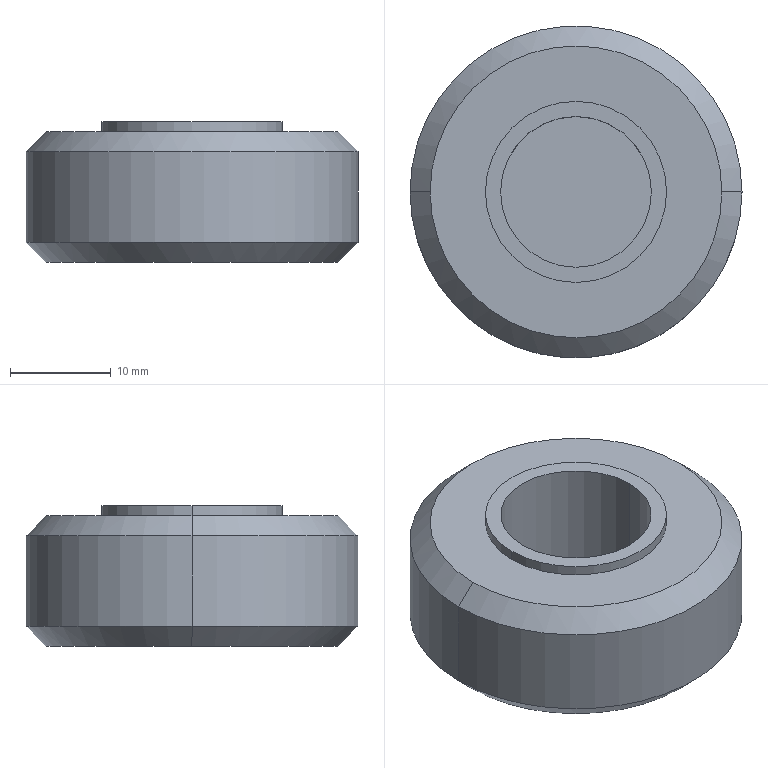Part | SolidWorks | features ICE 2, Chamfer 1, Extrusion 1 | 1 solid | 14 faces | box 33 x 33 x 14 mm | volume 9032 mm3 | cylinder 6 | cone 4 | plane 4 | commonest cylinder face diameters 15 x2 18 x2 33 x2
STEP:
#1=CARTESIAN_POINT('',(-14.5,0.,-3.));
#2=VERTEX_POINT('',#1);
#3=CARTESIAN_POINT('',(14.5,0.,-3.));
#4=VERTEX_POINT('',#3);
#5=CARTESIAN_POINT('',(0.,0.,-3.));
#6=DIRECTION('',(0.,0.,-1.));
#7=DIRECTION('',(-1.,0.,0.));
#8=AXIS2_PLACEMENT_3D('',#5,#6,#7);
#9=CIRCLE('',#8,14.5);
#10=EDGE_CURVE('',#2,#4,#9,.T.);
#11=ORIENTED_EDGE('',*,*,#10,.F.);
#12=CARTESIAN_POINT('',(-16.5,0.,-1.));
#13=VERTEX_POINT('',#12);
#14=CARTESIAN_POINT('',(-14.5,0.,-3.));
#15=DIRECTION('',(-0.7071,0.,0.7071));
#16=VECTOR('',#15,1000.);
#17=LINE('',#14,#16);
#18=EDGE_CURVE('',#2,#13,#17,.T.);
#19=ORIENTED_EDGE('',*,*,#18,.T.);
#20=CARTESIAN_POINT('',(16.5,0.,-1.));
#21=VERTEX_POINT('',#20);
#22=CARTESIAN_POINT('',(0.,0.,-1.));
#23=DIRECTION('',(0.,0.,1.));
#24=DIRECTION('',(-1.,0.,0.));
#25=AXIS2_PLACEMENT_3D('',#22,#23,#24);
#26=CIRCLE('',#25,16.5);
#27=EDGE_CURVE('',#21,#13,#26,.T.);
#28=ORIENTED_EDGE('',*,*,#27,.F.);
#29=CARTESIAN_POINT('',(14.5,0.,-3.));
#30=DIRECTION('',(0.7071,0.,0.7071));
#31=VECTOR('',#30,1000.);
#32=LINE('',#29,#31);
#33=EDGE_CURVE('',#4,#21,#32,.T.);
#34=ORIENTED_EDGE('',*,*,#33,.F.);
#35=EDGE_LOOP('',(#11,#19,#28,#34));
#36=FACE_OUTER_BOUND('',#35,.T.);
#37=CARTESIAN_POINT('',(0.,0.,-3.));
#38=DIRECTION('',(0.,0.,1.));
#39=DIRECTION('',(1.,0.,0.));
#40=AXIS2_PLACEMENT_3D('',#37,#38,#39);
#41=CONICAL_SURFACE('',#40,14.5,0.7854);
#42=ADVANCED_FACE('',(#36),#41,.T.);
#43=CARTESIAN_POINT('',(14.5,0.,10.));
#44=VERTEX_POINT('',#43);
#45=CARTESIAN_POINT('',(-14.5,0.,10.));
#46=VERTEX_POINT('',#45);
#47=CARTESIAN_POINT('',(0.,0.,10.));
#48=DIRECTION('',(0.,0.,1.));
#49=DIRECTION('',(1.,0.,0.));
#50=AXIS2_PLACEMENT_3D('',#47,#48,#49);
#51=CIRCLE('',#50,14.5);
#52=EDGE_CURVE('',#44,#46,#51,.T.);
#53=ORIENTED_EDGE('',*,*,#52,.F.);
#54=CARTESIAN_POINT('',(16.5,0.,8.));
#55=VERTEX_POINT('',#54);
#56=CARTESIAN_POINT('',(14.5,0.,10.));
#57=DIRECTION('',(0.7071,0.,-0.7071));
#58=VECTOR('',#57,1000.);
#59=LINE('',#56,#58);
#60=EDGE_CURVE('',#44,#55,#59,.T.);
#61=ORIENTED_EDGE('',*,*,#60,.T.);
#62=CARTESIAN_POINT('',(-16.5,0.,8.));
#63=VERTEX_POINT('',#62);
#64=CARTESIAN_POINT('',(0.,0.,8.));
#65=DIRECTION('',(0.,0.,-1.));
#66=DIRECTION('',(1.,0.,0.));
#67=AXIS2_PLACEMENT_3D('',#64,#65,#66);
#68=CIRCLE('',#67,16.5);
#69=EDGE_CURVE('',#63,#55,#68,.T.);
#70=ORIENTED_EDGE('',*,*,#69,.F.);
#71=CARTESIAN_POINT('',(-14.5,0.,10.));
#72=DIRECTION('',(-0.7071,0.,-0.7071));
#73=VECTOR('',#72,1000.);
#74=LINE('',#71,#73);
#75=EDGE_CURVE('',#46,#63,#74,.T.);
#76=ORIENTED_EDGE('',*,*,#75,.F.);
#77=EDGE_LOOP('',(#53,#61,#70,#76));
#78=FACE_OUTER_BOUND('',#77,.T.);
#79=CARTESIAN_POINT('',(0.,0.,10.));
#80=DIRECTION('',(0.,0.,-1.));
#81=DIRECTION('',(-1.,0.,0.));
#82=AXIS2_PLACEMENT_3D('',#79,#80,#81);
#83=CONICAL_SURFACE('',#82,14.5,0.7854);
#84=ADVANCED_FACE('',(#78),#83,.T.);
#85=CARTESIAN_POINT('',(9.,0.,11.));
#86=VERTEX_POINT('',#85);
#87=CARTESIAN_POINT('',(-9.,0.,11.));
#88=VERTEX_POINT('',#87);
#89=CARTESIAN_POINT('',(0.,0.,11.));
#90=DIRECTION('',(0.,0.,1.));
#91=DIRECTION('',(1.,0.,0.));
#92=AXIS2_PLACEMENT_3D('',#89,#90,#91);
#93=CIRCLE('',#92,9.);
#94=EDGE_CURVE('',#86,#88,#93,.T.);
#95=ORIENTED_EDGE('',*,*,#94,.F.);
#96=CARTESIAN_POINT('',(9.,0.,10.));
#97=VERTEX_POINT('',#96);
#98=CARTESIAN_POINT('',(9.,0.,11.));
#99=DIRECTION('',(0.,0.,-1.));
#100=VECTOR('',#99,1000.);
#101=LINE('',#98,#100);
#102=EDGE_CURVE('',#86,#97,#101,.T.);
#103=ORIENTED_EDGE('',*,*,#102,.T.);
#104=CARTESIAN_POINT('',(-9.,0.,10.));
#105=VERTEX_POINT('',#104);
#106=CARTESIAN_POINT('',(0.,0.,10.));
#107=DIRECTION('',(0.,0.,1.));
#108=DIRECTION('',(1.,0.,0.));
#109=AXIS2_PLACEMENT_3D('',#106,#107,#108);
#110=CIRCLE('',#109,9.);
#111=EDGE_CURVE('',#97,#105,#110,.T.);
#112=ORIENTED_EDGE('',*,*,#111,.T.);
#113=CARTESIAN_POINT('',(-9.,0.,11.));
#114=DIRECTION('',(0.,0.,-1.));
#115=VECTOR('',#114,1000.);
#116=LINE('',#113,#115);
#117=EDGE_CURVE('',#88,#105,#116,.T.);
#118=ORIENTED_EDGE('',*,*,#117,.F.);
#119=EDGE_LOOP('',(#95,#103,#112,#118));
#120=FACE_OUTER_BOUND('',#119,.T.);
#121=CARTESIAN_POINT('',(0.,0.,11.));
#122=DIRECTION('',(0.,0.,-1.));
#123=DIRECTION('',(-1.,0.,0.));
#124=AXIS2_PLACEMENT_3D('',#121,#122,#123);
#125=CYLINDRICAL_SURFACE('',#124,9.);
#126=ADVANCED_FACE('',(#120),#125,.T.);
#127=CARTESIAN_POINT('',(-7.5,0.,11.));
#128=VERTEX_POINT('',#127);
#129=CARTESIAN_POINT('',(7.5,0.,11.));
#130=VERTEX_POINT('',#129);
#131=CARTESIAN_POINT('',(0.,0.,11.));
#132=DIRECTION('',(0.,0.,1.));
#133=DIRECTION('',(1.,0.,0.));
#134=AXIS2_PLACEMENT_3D('',#131,#132,#133);
#135=CIRCLE('',#134,7.5);
#136=EDGE_CURVE('',#128,#130,#135,.T.);
#137=ORIENTED_EDGE('',*,*,#136,.T.);
#138=CARTESIAN_POINT('',(7.5,0.,0.));
#139=VERTEX_POINT('',#138);
#140=CARTESIAN_POINT('',(7.5,0.,10.));
#141=DIRECTION('',(0.,0.,-1.));
#142=VECTOR('',#141,1000.);
#143=LINE('',#140,#142);
#144=EDGE_CURVE('',#130,#139,#143,.T.);
#145=ORIENTED_EDGE('',*,*,#144,.T.);
#146=CARTESIAN_POINT('',(-7.5,0.,0.));
#147=VERTEX_POINT('',#146);
#148=CARTESIAN_POINT('',(0.,0.,0.));
#149=DIRECTION('',(0.,0.,1.));
#150=DIRECTION('',(1.,0.,0.));
#151=AXIS2_PLACEMENT_3D('',#148,#149,#150);
#152=CIRCLE('',#151,7.5);
#153=EDGE_CURVE('',#147,#139,#152,.T.);
#154=ORIENTED_EDGE('',*,*,#153,.F.);
#155=CARTESIAN_POINT('',(-7.5,0.,10.));
#156=DIRECTION('',(0.,0.,-1.));
#157=VECTOR('',#156,1000.);
#158=LINE('',#155,#157);
#159=EDGE_CURVE('',#128,#147,#158,.T.);
#160=ORIENTED_EDGE('',*,*,#159,.F.);
#161=EDGE_LOOP('',(#137,#145,#154,#160));
#162=FACE_OUTER_BOUND('',#161,.T.);
#163=CARTESIAN_POINT('',(0.,0.,10.));
#164=DIRECTION('',(0.,0.,-1.));
#165=DIRECTION('',(-1.,0.,0.));
#166=AXIS2_PLACEMENT_3D('',#163,#164,#165);
#167=CYLINDRICAL_SURFACE('',#166,7.5);
#168=ADVANCED_FACE('',(#162),#167,.F.);
#169=ORIENTED_EDGE('',*,*,#69,.T.);
#170=CARTESIAN_POINT('',(16.5,0.,10.));
#171=DIRECTION('',(0.,0.,-1.));
#172=VECTOR('',#171,1000.);
#173=LINE('',#170,#172);
#174=EDGE_CURVE('',#55,#21,#173,.T.);
#175=ORIENTED_EDGE('',*,*,#174,.T.);
#176=ORIENTED_EDGE('',*,*,#27,.T.);
#177=CARTESIAN_POINT('',(-16.5,0.,10.));
#178=DIRECTION('',(0.,0.,-1.));
#179=VECTOR('',#178,1000.);
#180=LINE('',#177,#179);
#181=EDGE_CURVE('',#63,#13,#180,.T.);
#182=ORIENTED_EDGE('',*,*,#181,.F.);
#183=EDGE_LOOP('',(#169,#175,#176,#182));
#184=FACE_OUTER_BOUND('',#183,.T.);
#185=CARTESIAN_POINT('',(0.,0.,10.));
#186=DIRECTION('',(0.,0.,-1.));
#187=DIRECTION('',(-1.,0.,0.));
#188=AXIS2_PLACEMENT_3D('',#185,#186,#187);
#189=CYLINDRICAL_SURFACE('',#188,16.5);
#190=ADVANCED_FACE('',(#184),#189,.T.);
#191=CARTESIAN_POINT('',(0.,0.,10.));
#192=DIRECTION('',(0.,0.,1.));
#193=DIRECTION('',(1.,0.,0.));
#194=AXIS2_PLACEMENT_3D('',#191,#192,#193);
#195=CIRCLE('',#194,14.5);
#196=EDGE_CURVE('',#46,#44,#195,.T.);
#197=ORIENTED_EDGE('',*,*,#196,.T.);
#198=ORIENTED_EDGE('',*,*,#52,.T.);
#199=EDGE_LOOP('',(#197,#198));
#200=FACE_OUTER_BOUND('',#199,.T.);
#201=CARTESIAN_POINT('',(0.,0.,10.));
#202=DIRECTION('',(0.,0.,1.));
#203=DIRECTION('',(1.,0.,0.));
#204=AXIS2_PLACEMENT_3D('',#201,#202,#203);
#205=CIRCLE('',#204,9.);
#206=EDGE_CURVE('',#105,#97,#205,.T.);
#207=ORIENTED_EDGE('',*,*,#206,.F.);
#208=ORIENTED_EDGE('',*,*,#111,.F.);
#209=EDGE_LOOP('',(#207,#208));
#210=FACE_BOUND('',#209,.T.);
#211=CARTESIAN_POINT('',(0.,0.,10.));
#212=DIRECTION('',(0.,0.,1.));
#213=DIRECTION('',(1.,0.,0.));
#214=AXIS2_PLACEMENT_3D('',#211,#212,#213);
#215=PLANE('',#214);
#216=ADVANCED_FACE('',(#200,#210),#215,.T.);
#217=ORIENTED_EDGE('',*,*,#174,.F.);
#218=CARTESIAN_POINT('',(0.,0.,8.));
#219=DIRECTION('',(0.,0.,-1.));
#220=DIRECTION('',(1.,0.,0.));
#221=AXIS2_PLACEMENT_3D('',#218,#219,#220);
#222=CIRCLE('',#221,16.5);
#223=EDGE_CURVE('',#55,#63,#222,.T.);
#224=ORIENTED_EDGE('',*,*,#223,.T.);
#225=ORIENTED_EDGE('',*,*,#181,.T.);
#226=CARTESIAN_POINT('',(0.,0.,-1.));
#227=DIRECTION('',(0.,0.,1.));
#228=DIRECTION('',(-1.,0.,0.));
#229=AXIS2_PLACEMENT_3D('',#226,#227,#228);
#230=CIRCLE('',#229,16.5);
#231=EDGE_CURVE('',#13,#21,#230,.T.);
#232=ORIENTED_EDGE('',*,*,#231,.T.);
#233=EDGE_LOOP('',(#217,#224,#225,#232));
#234=FACE_OUTER_BOUND('',#233,.T.);
#235=CARTESIAN_POINT('',(0.,0.,10.));
#236=DIRECTION('',(0.,0.,-1.));
#237=DIRECTION('',(-1.,0.,0.));
#238=AXIS2_PLACEMENT_3D('',#235,#236,#237);
#239=CYLINDRICAL_SURFACE('',#238,16.5);
#240=ADVANCED_FACE('',(#234),#239,.T.);
#241=ORIENTED_EDGE('',*,*,#144,.F.);
#242=CARTESIAN_POINT('',(0.,0.,11.));
#243=DIRECTION('',(0.,0.,1.));
#244=DIRECTION('',(1.,0.,0.));
#245=AXIS2_PLACEMENT_3D('',#242,#243,#244);
#246=CIRCLE('',#245,7.5);
#247=EDGE_CURVE('',#130,#128,#246,.T.);
#248=ORIENTED_EDGE('',*,*,#247,.T.);
#249=ORIENTED_EDGE('',*,*,#159,.T.);
#250=CARTESIAN_POINT('',(0.,0.,0.));
#251=DIRECTION('',(0.,0.,1.));
#252=DIRECTION('',(1.,0.,0.));
#253=AXIS2_PLACEMENT_3D('',#250,#251,#252);
#254=CIRCLE('',#253,7.5);
#255=EDGE_CURVE('',#139,#147,#254,.T.);
#256=ORIENTED_EDGE('',*,*,#255,.F.);
#257=EDGE_LOOP('',(#241,#248,#249,#256));
#258=FACE_OUTER_BOUND('',#257,.T.);
#259=CARTESIAN_POINT('',(0.,0.,10.));
#260=DIRECTION('',(0.,0.,-1.));
#261=DIRECTION('',(-1.,0.,0.));
#262=AXIS2_PLACEMENT_3D('',#259,#260,#261);
#263=CYLINDRICAL_SURFACE('',#262,7.5);
#264=ADVANCED_FACE('',(#258),#263,.F.);
#265=CARTESIAN_POINT('',(0.,0.,11.));
#266=DIRECTION('',(0.,0.,1.));
#267=DIRECTION('',(1.,0.,0.));
#268=AXIS2_PLACEMENT_3D('',#265,#266,#267);
#269=CIRCLE('',#268,9.);
#270=EDGE_CURVE('',#88,#86,#269,.T.);
#271=ORIENTED_EDGE('',*,*,#270,.T.);
#272=ORIENTED_EDGE('',*,*,#94,.T.);
#273=EDGE_LOOP('',(#271,#272));
#274=FACE_OUTER_BOUND('',#273,.T.);
#275=ORIENTED_EDGE('',*,*,#136,.F.);
#276=ORIENTED_EDGE('',*,*,#247,.F.);
#277=EDGE_LOOP('',(#275,#276));
#278=FACE_BOUND('',#277,.T.);
#279=CARTESIAN_POINT('',(0.,0.,11.));
#280=DIRECTION('',(0.,0.,1.));
#281=DIRECTION('',(1.,0.,0.));
#282=AXIS2_PLACEMENT_3D('',#279,#280,#281);
#283=PLANE('',#282);
#284=ADVANCED_FACE('',(#274,#278),#283,.T.);
#285=ORIENTED_EDGE('',*,*,#102,.F.);
#286=ORIENTED_EDGE('',*,*,#270,.F.);
#287=ORIENTED_EDGE('',*,*,#117,.T.);
#288=ORIENTED_EDGE('',*,*,#206,.T.);
#289=EDGE_LOOP('',(#285,#286,#287,#288));
#290=FACE_OUTER_BOUND('',#289,.T.);
#291=CARTESIAN_POINT('',(0.,0.,11.));
#292=DIRECTION('',(0.,0.,-1.));
#293=DIRECTION('',(-1.,0.,0.));
#294=AXIS2_PLACEMENT_3D('',#291,#292,#293);
#295=CYLINDRICAL_SURFACE('',#294,9.);
#296=ADVANCED_FACE('',(#290),#295,.T.);
#297=ORIENTED_EDGE('',*,*,#153,.T.);
#298=ORIENTED_EDGE('',*,*,#255,.T.);
#299=EDGE_LOOP('',(#297,#298));
#300=FACE_OUTER_BOUND('',#299,.T.);
#301=CARTESIAN_POINT('',(0.,0.,0.));
#302=DIRECTION('',(0.,0.,-1.));
#303=DIRECTION('',(-1.,0.,0.));
#304=AXIS2_PLACEMENT_3D('',#301,#302,#303);
#305=PLANE('',#304);
#306=ADVANCED_FACE('',(#300),#305,.F.);
#307=CARTESIAN_POINT('',(0.,0.,-3.));
#308=DIRECTION('',(0.,0.,-1.));
#309=DIRECTION('',(-1.,0.,0.));
#310=AXIS2_PLACEMENT_3D('',#307,#308,#309);
#311=CIRCLE('',#310,14.5);
#312=EDGE_CURVE('',#4,#2,#311,.T.);
#313=ORIENTED_EDGE('',*,*,#312,.T.);
#314=ORIENTED_EDGE('',*,*,#10,.T.);
#315=EDGE_LOOP('',(#313,#314));
#316=FACE_OUTER_BOUND('',#315,.T.);
#317=CARTESIAN_POINT('',(0.,0.,-3.));
#318=DIRECTION('',(0.,0.,-1.));
#319=DIRECTION('',(-1.,0.,0.));
#320=AXIS2_PLACEMENT_3D('',#317,#318,#319);
#321=PLANE('',#320);
#322=ADVANCED_FACE('',(#316),#321,.T.);
#323=ORIENTED_EDGE('',*,*,#60,.F.);
#324=ORIENTED_EDGE('',*,*,#196,.F.);
#325=ORIENTED_EDGE('',*,*,#75,.T.);
#326=ORIENTED_EDGE('',*,*,#223,.F.);
#327=EDGE_LOOP('',(#323,#324,#325,#326));
#328=FACE_OUTER_BOUND('',#327,.T.);
#329=CARTESIAN_POINT('',(0.,0.,10.));
#330=DIRECTION('',(0.,0.,-1.));
#331=DIRECTION('',(-1.,0.,0.));
#332=AXIS2_PLACEMENT_3D('',#329,#330,#331);
#333=CONICAL_SURFACE('',#332,14.5,0.7854);
#334=ADVANCED_FACE('',(#328),#333,.T.);
#335=ORIENTED_EDGE('',*,*,#18,.F.);
#336=ORIENTED_EDGE('',*,*,#312,.F.);
#337=ORIENTED_EDGE('',*,*,#33,.T.);
#338=ORIENTED_EDGE('',*,*,#231,.F.);
#339=EDGE_LOOP('',(#335,#336,#337,#338));
#340=FACE_OUTER_BOUND('',#339,.T.);
#341=CARTESIAN_POINT('',(0.,0.,-3.));
#342=DIRECTION('',(0.,0.,1.));
#343=DIRECTION('',(1.,0.,0.));
#344=AXIS2_PLACEMENT_3D('',#341,#342,#343);
#345=CONICAL_SURFACE('',#344,14.5,0.7854);
#346=ADVANCED_FACE('',(#340),#345,.T.);
#347=CLOSED_SHELL('',(#42,#84,#126,#168,#190,#216,#240,#264,#284,#296,#306,#322,#334,#346));
#348=MANIFOLD_SOLID_BREP('',#347);
#349=CARTESIAN_POINT('',(0.,0.,0.));
#350=DIRECTION('',(0.,0.,1.));
#351=DIRECTION('',(1.,0.,0.));
#352=AXIS2_PLACEMENT_3D('',#349,#350,#351);
#353=(LENGTH_UNIT()NAMED_UNIT(*)SI_UNIT(.MILLI.,.METRE.));
#354=UNCERTAINTY_MEASURE_WITH_UNIT(LENGTH_MEASURE(0.00001),#353,'','');
#355=(NAMED_UNIT(*)PLANE_ANGLE_UNIT()SI_UNIT($,.RADIAN.));
#356=(NAMED_UNIT(*)SI_UNIT($,.STERADIAN.)SOLID_ANGLE_UNIT());
#357=(GEOMETRIC_REPRESENTATION_CONTEXT(3)GLOBAL_UNCERTAINTY_ASSIGNED_CONTEXT((#354))GLOBAL_UNIT_ASSIGNED_CONTEXT((#353,#355,#356))REPRESENTATION_CONTEXT('',''));
#358=ADVANCED_BREP_SHAPE_REPRESENTATION('',(#348,#352),#357);